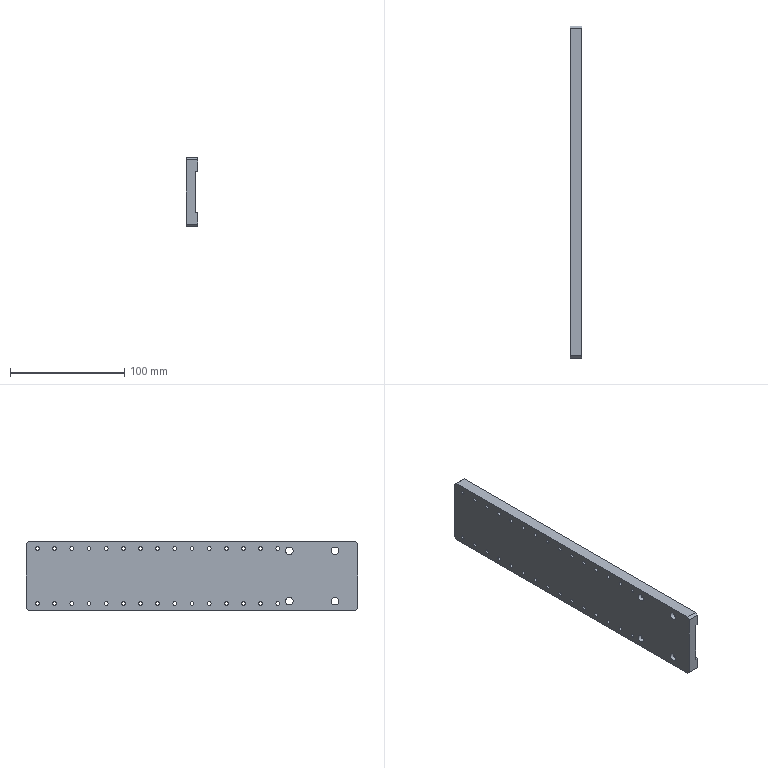Part | NX | 1 solid | 60 faces | box 10 x 290 x 60 mm | volume 147611 mm3 | cylinder 38 | plane 22 | commonest cylinder face diameters 3.3 x30 6.6 x4 11 x4